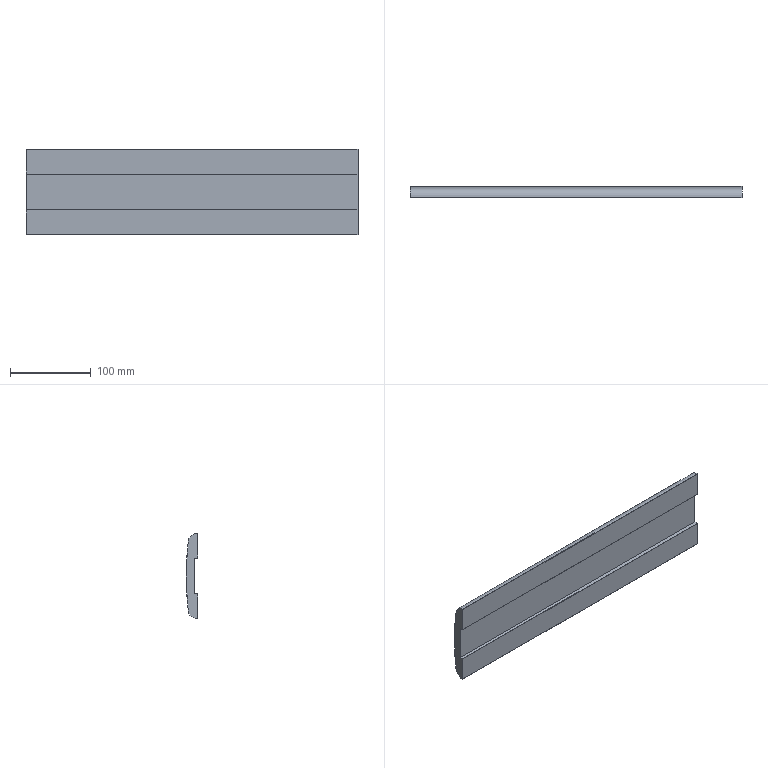Part | SolidWorks | features BaseBody 1 | 1 solid | 31 faces | box 411 x 14.5 x 106.047 mm | volume 473016 mm3 | cylinder 22 | plane 9 | commonest cylinder face diameters 0.2 x8 0.6 x6 22 x3 660 x3 0.4 x2
STEP:
#1=CARTESIAN_POINT('',(0.,60.288,-53.015));
#2=VERTEX_POINT('',#1);
#3=CARTESIAN_POINT('',(0.,60.72,-53.023));
#4=VERTEX_POINT('',#3);
#5=CARTESIAN_POINT('',(0.,60.72,-42.023));
#6=DIRECTION('',(1.,0.,0.));
#7=DIRECTION('',(0.,0.,-1.));
#8=AXIS2_PLACEMENT_3D('',#5,#6,#7);
#9=CIRCLE('',#8,11.);
#10=EDGE_CURVE('',#2,#4,#9,.T.);
#11=ORIENTED_EDGE('',*,*,#10,.T.);
#12=CARTESIAN_POINT('',(411.,60.72,-53.023));
#13=VERTEX_POINT('',#12);
#14=CARTESIAN_POINT('',(411.,60.72,-53.023));
#15=DIRECTION('',(1.,0.,0.));
#16=VECTOR('',#15,1000.);
#17=LINE('',#14,#16);
#18=EDGE_CURVE('',#4,#13,#17,.T.);
#19=ORIENTED_EDGE('',*,*,#18,.T.);
#20=CARTESIAN_POINT('',(411.,60.288,-53.015));
#21=VERTEX_POINT('',#20);
#22=CARTESIAN_POINT('',(411.,60.72,-42.023));
#23=DIRECTION('',(1.,0.,0.));
#24=DIRECTION('',(0.,0.,-1.));
#25=AXIS2_PLACEMENT_3D('',#22,#23,#24);
#26=CIRCLE('',#25,11.);
#27=EDGE_CURVE('',#21,#13,#26,.T.);
#28=ORIENTED_EDGE('',*,*,#27,.F.);
#29=CARTESIAN_POINT('',(411.,60.288,-53.015));
#30=DIRECTION('',(-1.,0.,0.));
#31=VECTOR('',#30,1000.);
#32=LINE('',#29,#31);
#33=EDGE_CURVE('',#21,#2,#32,.T.);
#34=ORIENTED_EDGE('',*,*,#33,.T.);
#35=EDGE_LOOP('',(#11,#19,#28,#34));
#36=FACE_OUTER_BOUND('',#35,.T.);
#37=CARTESIAN_POINT('',(411.,60.72,-42.023));
#38=DIRECTION('',(1.,0.,0.));
#39=DIRECTION('',(0.,0.,-1.));
#40=AXIS2_PLACEMENT_3D('',#37,#38,#39);
#41=CYLINDRICAL_SURFACE('',#40,11.);
#42=ADVANCED_FACE('',(#36),#41,.T.);
#43=CARTESIAN_POINT('',(411.,73.654,23.614));
#44=VERTEX_POINT('',#43);
#45=CARTESIAN_POINT('',(411.,73.654,-23.614));
#46=VERTEX_POINT('',#45);
#47=CARTESIAN_POINT('',(411.,-255.5,0.));
#48=DIRECTION('',(-1.,0.,0.));
#49=DIRECTION('',(0.,0.,-1.));
#50=AXIS2_PLACEMENT_3D('',#47,#48,#49);
#51=CIRCLE('',#50,330.);
#52=EDGE_CURVE('',#44,#46,#51,.T.);
#53=ORIENTED_EDGE('',*,*,#52,.T.);
#54=CARTESIAN_POINT('',(0.,73.654,-23.614));
#55=VERTEX_POINT('',#54);
#56=CARTESIAN_POINT('',(411.,73.654,-23.614));
#57=DIRECTION('',(-1.,0.,0.));
#58=VECTOR('',#57,1000.);
#59=LINE('',#56,#58);
#60=EDGE_CURVE('',#46,#55,#59,.T.);
#61=ORIENTED_EDGE('',*,*,#60,.T.);
#62=CARTESIAN_POINT('',(0.,73.654,23.614));
#63=VERTEX_POINT('',#62);
#64=CARTESIAN_POINT('',(0.,-255.5,0.));
#65=DIRECTION('',(1.,0.,0.));
#66=DIRECTION('',(0.,0.,-1.));
#67=AXIS2_PLACEMENT_3D('',#64,#65,#66);
#68=CIRCLE('',#67,330.);
#69=EDGE_CURVE('',#55,#63,#68,.T.);
#70=ORIENTED_EDGE('',*,*,#69,.T.);
#71=CARTESIAN_POINT('',(411.,73.654,23.614));
#72=DIRECTION('',(1.,0.,0.));
#73=VECTOR('',#72,1000.);
#74=LINE('',#71,#73);
#75=EDGE_CURVE('',#63,#44,#74,.T.);
#76=ORIENTED_EDGE('',*,*,#75,.T.);
#77=EDGE_LOOP('',(#53,#61,#70,#76));
#78=FACE_OUTER_BOUND('',#77,.T.);
#79=CARTESIAN_POINT('',(411.,-255.5,0.));
#80=DIRECTION('',(1.,0.,0.));
#81=DIRECTION('',(0.,0.,-1.));
#82=AXIS2_PLACEMENT_3D('',#79,#80,#81);
#83=CYLINDRICAL_SURFACE('',#82,330.);
#84=ADVANCED_FACE('',(#78),#83,.T.);
#85=CARTESIAN_POINT('',(411.,73.572,-23.705));
#86=VERTEX_POINT('',#85);
#87=CARTESIAN_POINT('',(411.,73.554,-23.607));
#88=DIRECTION('',(-1.,0.,0.));
#89=DIRECTION('',(0.,0.,-1.));
#90=AXIS2_PLACEMENT_3D('',#87,#88,#89);
#91=CIRCLE('',#90,0.1);
#92=EDGE_CURVE('',#46,#86,#91,.T.);
#93=ORIENTED_EDGE('',*,*,#92,.T.);
#94=CARTESIAN_POINT('',(0.,73.572,-23.705));
#95=VERTEX_POINT('',#94);
#96=CARTESIAN_POINT('',(411.,73.572,-23.705));
#97=DIRECTION('',(-1.,0.,0.));
#98=VECTOR('',#97,1000.);
#99=LINE('',#96,#98);
#100=EDGE_CURVE('',#86,#95,#99,.T.);
#101=ORIENTED_EDGE('',*,*,#100,.T.);
#102=CARTESIAN_POINT('',(0.,73.554,-23.607));
#103=DIRECTION('',(1.,0.,0.));
#104=DIRECTION('',(0.,0.,-1.));
#105=AXIS2_PLACEMENT_3D('',#102,#103,#104);
#106=CIRCLE('',#105,0.1);
#107=EDGE_CURVE('',#95,#55,#106,.T.);
#108=ORIENTED_EDGE('',*,*,#107,.T.);
#109=ORIENTED_EDGE('',*,*,#60,.F.);
#110=EDGE_LOOP('',(#93,#101,#108,#109));
#111=FACE_OUTER_BOUND('',#110,.T.);
#112=CARTESIAN_POINT('',(411.,73.554,-23.607));
#113=DIRECTION('',(1.,0.,0.));
#114=DIRECTION('',(0.,0.,-1.));
#115=AXIS2_PLACEMENT_3D('',#112,#113,#114);
#116=CYLINDRICAL_SURFACE('',#115,0.1);
#117=ADVANCED_FACE('',(#111),#116,.T.);
#118=CARTESIAN_POINT('',(411.,73.499,24.705));
#119=VERTEX_POINT('',#118);
#120=CARTESIAN_POINT('',(411.,73.455,25.284));
#121=VERTEX_POINT('',#120);
#122=CARTESIAN_POINT('',(411.,73.552,25.));
#123=DIRECTION('',(-1.,0.,0.));
#124=DIRECTION('',(0.,0.,-1.));
#125=AXIS2_PLACEMENT_3D('',#122,#123,#124);
#126=CIRCLE('',#125,0.3);
#127=EDGE_CURVE('',#119,#121,#126,.T.);
#128=ORIENTED_EDGE('',*,*,#127,.T.);
#129=CARTESIAN_POINT('',(411.,73.522,25.386));
#130=VERTEX_POINT('',#129);
#131=CARTESIAN_POINT('',(411.,73.422,25.378));
#132=DIRECTION('',(-1.,0.,0.));
#133=DIRECTION('',(0.,0.,-1.));
#134=AXIS2_PLACEMENT_3D('',#131,#132,#133);
#135=CIRCLE('',#134,0.1);
#136=EDGE_CURVE('',#130,#121,#135,.T.);
#137=ORIENTED_EDGE('',*,*,#136,.F.);
#138=CARTESIAN_POINT('',(411.,71.624,43.473));
#139=VERTEX_POINT('',#138);
#140=CARTESIAN_POINT('',(411.,-255.5,0.002391));
#141=DIRECTION('',(1.,0.,0.));
#142=DIRECTION('',(0.,0.,-1.));
#143=AXIS2_PLACEMENT_3D('',#140,#141,#142);
#144=CIRCLE('',#143,330.);
#145=EDGE_CURVE('',#130,#139,#144,.T.);
#146=ORIENTED_EDGE('',*,*,#145,.T.);
#147=CARTESIAN_POINT('',(411.,60.288,53.015));
#148=VERTEX_POINT('',#147);
#149=CARTESIAN_POINT('',(411.,60.72,42.023));
#150=DIRECTION('',(1.,0.,0.));
#151=DIRECTION('',(0.,0.,-1.));
#152=AXIS2_PLACEMENT_3D('',#149,#150,#151);
#153=CIRCLE('',#152,11.);
#154=EDGE_CURVE('',#139,#148,#153,.T.);
#155=ORIENTED_EDGE('',*,*,#154,.T.);
#156=CARTESIAN_POINT('',(411.,60.,52.715));
#157=VERTEX_POINT('',#156);
#158=CARTESIAN_POINT('',(411.,60.3,52.715));
#159=DIRECTION('',(-1.,0.,0.));
#160=DIRECTION('',(0.,0.,-1.));
#161=AXIS2_PLACEMENT_3D('',#158,#159,#160);
#162=CIRCLE('',#161,0.3);
#163=EDGE_CURVE('',#157,#148,#162,.T.);
#164=ORIENTED_EDGE('',*,*,#163,.F.);
#165=CARTESIAN_POINT('',(411.,60.,22.2));
#166=VERTEX_POINT('',#165);
#167=CARTESIAN_POINT('',(411.,60.,0.002391));
#168=DIRECTION('',(0.,0.,-1.));
#169=VECTOR('',#168,1000.);
#170=LINE('',#167,#169);
#171=EDGE_CURVE('',#157,#166,#170,.T.);
#172=ORIENTED_EDGE('',*,*,#171,.T.);
#173=CARTESIAN_POINT('',(411.,60.2,22.));
#174=VERTEX_POINT('',#173);
#175=CARTESIAN_POINT('',(411.,60.2,22.2));
#176=DIRECTION('',(-1.,0.,0.));
#177=DIRECTION('',(0.,0.,-1.));
#178=AXIS2_PLACEMENT_3D('',#175,#176,#177);
#179=CIRCLE('',#178,0.2);
#180=EDGE_CURVE('',#174,#166,#179,.T.);
#181=ORIENTED_EDGE('',*,*,#180,.F.);
#182=CARTESIAN_POINT('',(411.,64.5,22.));
#183=VERTEX_POINT('',#182);
#184=CARTESIAN_POINT('',(411.,-255.5,22.));
#185=DIRECTION('',(0.,1.,0.));
#186=VECTOR('',#185,1000.);
#187=LINE('',#184,#186);
#188=EDGE_CURVE('',#174,#183,#187,.T.);
#189=ORIENTED_EDGE('',*,*,#188,.T.);
#190=CARTESIAN_POINT('',(411.,64.5,-22.));
#191=VERTEX_POINT('',#190);
#192=CARTESIAN_POINT('',(411.,64.5,0.002391));
#193=DIRECTION('',(0.,0.,-1.));
#194=VECTOR('',#193,1000.);
#195=LINE('',#192,#194);
#196=EDGE_CURVE('',#183,#191,#195,.T.);
#197=ORIENTED_EDGE('',*,*,#196,.T.);
#198=CARTESIAN_POINT('',(411.,60.2,-22.));
#199=VERTEX_POINT('',#198);
#200=CARTESIAN_POINT('',(411.,-255.5,-22.));
#201=DIRECTION('',(0.,-1.,0.));
#202=VECTOR('',#201,1000.);
#203=LINE('',#200,#202);
#204=EDGE_CURVE('',#191,#199,#203,.T.);
#205=ORIENTED_EDGE('',*,*,#204,.T.);
#206=CARTESIAN_POINT('',(411.,60.,-22.2));
#207=VERTEX_POINT('',#206);
#208=CARTESIAN_POINT('',(411.,60.2,-22.2));
#209=DIRECTION('',(-1.,0.,0.));
#210=DIRECTION('',(0.,0.,-1.));
#211=AXIS2_PLACEMENT_3D('',#208,#209,#210);
#212=CIRCLE('',#211,0.2);
#213=EDGE_CURVE('',#207,#199,#212,.T.);
#214=ORIENTED_EDGE('',*,*,#213,.F.);
#215=CARTESIAN_POINT('',(411.,60.,-52.715));
#216=VERTEX_POINT('',#215);
#217=CARTESIAN_POINT('',(411.,60.,0.002391));
#218=DIRECTION('',(0.,0.,-1.));
#219=VECTOR('',#218,1000.);
#220=LINE('',#217,#219);
#221=EDGE_CURVE('',#207,#216,#220,.T.);
#222=ORIENTED_EDGE('',*,*,#221,.T.);
#223=CARTESIAN_POINT('',(411.,60.3,-52.715));
#224=DIRECTION('',(-1.,0.,0.));
#225=DIRECTION('',(0.,0.,-1.));
#226=AXIS2_PLACEMENT_3D('',#223,#224,#225);
#227=CIRCLE('',#226,0.3);
#228=EDGE_CURVE('',#21,#216,#227,.T.);
#229=ORIENTED_EDGE('',*,*,#228,.F.);
#230=ORIENTED_EDGE('',*,*,#27,.T.);
#231=CARTESIAN_POINT('',(411.,71.624,-43.473));
#232=VERTEX_POINT('',#231);
#233=CARTESIAN_POINT('',(411.,60.72,-42.023));
#234=DIRECTION('',(1.,0.,0.));
#235=DIRECTION('',(0.,0.,-1.));
#236=AXIS2_PLACEMENT_3D('',#233,#234,#235);
#237=CIRCLE('',#236,11.);
#238=EDGE_CURVE('',#13,#232,#237,.T.);
#239=ORIENTED_EDGE('',*,*,#238,.T.);
#240=CARTESIAN_POINT('',(411.,73.522,-25.386));
#241=VERTEX_POINT('',#240);
#242=CARTESIAN_POINT('',(411.,-255.5,-0.002391));
#243=DIRECTION('',(1.,0.,0.));
#244=DIRECTION('',(0.,0.,-1.));
#245=AXIS2_PLACEMENT_3D('',#242,#243,#244);
#246=CIRCLE('',#245,330.);
#247=EDGE_CURVE('',#232,#241,#246,.T.);
#248=ORIENTED_EDGE('',*,*,#247,.T.);
#249=CARTESIAN_POINT('',(411.,73.455,-25.284));
#250=VERTEX_POINT('',#249);
#251=CARTESIAN_POINT('',(411.,73.422,-25.378));
#252=DIRECTION('',(-1.,0.,0.));
#253=DIRECTION('',(0.,0.,-1.));
#254=AXIS2_PLACEMENT_3D('',#251,#252,#253);
#255=CIRCLE('',#254,0.1);
#256=EDGE_CURVE('',#250,#241,#255,.T.);
#257=ORIENTED_EDGE('',*,*,#256,.F.);
#258=CARTESIAN_POINT('',(411.,73.499,-24.705));
#259=VERTEX_POINT('',#258);
#260=CARTESIAN_POINT('',(411.,73.552,-25.));
#261=DIRECTION('',(-1.,0.,0.));
#262=DIRECTION('',(0.,0.,-1.));
#263=AXIS2_PLACEMENT_3D('',#260,#261,#262);
#264=CIRCLE('',#263,0.3);
#265=EDGE_CURVE('',#250,#259,#264,.T.);
#266=ORIENTED_EDGE('',*,*,#265,.T.);
#267=CARTESIAN_POINT('',(411.,73.581,-24.614));
#268=VERTEX_POINT('',#267);
#269=CARTESIAN_POINT('',(411.,73.481,-24.607));
#270=DIRECTION('',(-1.,0.,0.));
#271=DIRECTION('',(0.,0.,-1.));
#272=AXIS2_PLACEMENT_3D('',#269,#270,#271);
#273=CIRCLE('',#272,0.1);
#274=EDGE_CURVE('',#268,#259,#273,.T.);
#275=ORIENTED_EDGE('',*,*,#274,.F.);
#276=CARTESIAN_POINT('',(411.,73.598,-24.386));
#277=VERTEX_POINT('',#276);
#278=CARTESIAN_POINT('',(411.,73.581,-24.614));
#279=DIRECTION('',(0.,0.07436,0.9972));
#280=VECTOR('',#279,1000.);
#281=LINE('',#278,#280);
#282=EDGE_CURVE('',#268,#277,#281,.T.);
#283=ORIENTED_EDGE('',*,*,#282,.T.);
#284=CARTESIAN_POINT('',(411.,73.53,-24.284));
#285=VERTEX_POINT('',#284);
#286=CARTESIAN_POINT('',(411.,73.498,-24.379));
#287=DIRECTION('',(-1.,0.,0.));
#288=DIRECTION('',(0.,0.,-1.));
#289=AXIS2_PLACEMENT_3D('',#286,#287,#288);
#290=CIRCLE('',#289,0.1);
#291=EDGE_CURVE('',#285,#277,#290,.T.);
#292=ORIENTED_EDGE('',*,*,#291,.F.);
#293=CARTESIAN_POINT('',(411.,73.627,-24.));
#294=DIRECTION('',(-1.,0.,0.));
#295=DIRECTION('',(0.,0.,-1.));
#296=AXIS2_PLACEMENT_3D('',#293,#294,#295);
#297=CIRCLE('',#296,0.3);
#298=EDGE_CURVE('',#285,#86,#297,.T.);
#299=ORIENTED_EDGE('',*,*,#298,.T.);
#300=ORIENTED_EDGE('',*,*,#92,.F.);
#301=ORIENTED_EDGE('',*,*,#52,.F.);
#302=CARTESIAN_POINT('',(411.,73.572,23.705));
#303=VERTEX_POINT('',#302);
#304=CARTESIAN_POINT('',(411.,73.554,23.607));
#305=DIRECTION('',(1.,0.,0.));
#306=DIRECTION('',(0.,0.,-1.));
#307=AXIS2_PLACEMENT_3D('',#304,#305,#306);
#308=CIRCLE('',#307,0.1);
#309=EDGE_CURVE('',#44,#303,#308,.T.);
#310=ORIENTED_EDGE('',*,*,#309,.T.);
#311=CARTESIAN_POINT('',(411.,73.53,24.284));
#312=VERTEX_POINT('',#311);
#313=CARTESIAN_POINT('',(411.,73.627,24.));
#314=DIRECTION('',(-1.,0.,0.));
#315=DIRECTION('',(0.,0.,-1.));
#316=AXIS2_PLACEMENT_3D('',#313,#314,#315);
#317=CIRCLE('',#316,0.3);
#318=EDGE_CURVE('',#303,#312,#317,.T.);
#319=ORIENTED_EDGE('',*,*,#318,.T.);
#320=CARTESIAN_POINT('',(411.,73.598,24.386));
#321=VERTEX_POINT('',#320);
#322=CARTESIAN_POINT('',(411.,73.498,24.379));
#323=DIRECTION('',(-1.,0.,0.));
#324=DIRECTION('',(0.,0.,-1.));
#325=AXIS2_PLACEMENT_3D('',#322,#323,#324);
#326=CIRCLE('',#325,0.1);
#327=EDGE_CURVE('',#321,#312,#326,.T.);
#328=ORIENTED_EDGE('',*,*,#327,.F.);
#329=CARTESIAN_POINT('',(411.,73.581,24.614));
#330=VERTEX_POINT('',#329);
#331=CARTESIAN_POINT('',(411.,73.598,24.386));
#332=DIRECTION('',(0.,-0.07436,0.9972));
#333=VECTOR('',#332,1000.);
#334=LINE('',#331,#333);
#335=EDGE_CURVE('',#321,#330,#334,.T.);
#336=ORIENTED_EDGE('',*,*,#335,.T.);
#337=CARTESIAN_POINT('',(411.,73.481,24.607));
#338=DIRECTION('',(-1.,0.,0.));
#339=DIRECTION('',(0.,0.,-1.));
#340=AXIS2_PLACEMENT_3D('',#337,#338,#339);
#341=CIRCLE('',#340,0.1);
#342=EDGE_CURVE('',#119,#330,#341,.T.);
#343=ORIENTED_EDGE('',*,*,#342,.F.);
#344=EDGE_LOOP('',(#128,#137,#146,#155,#164,#172,#181,#189,#197,#205,#214,#222,#229,#230,#239,#248,#257,#266,#275,#283,#292,#299,#300,#301,#310,#319,#328,#336,#343));
#345=FACE_OUTER_BOUND('',#344,.T.);
#346=CARTESIAN_POINT('',(411.,-255.5,0.002391));
#347=DIRECTION('',(1.,0.,0.));
#348=DIRECTION('',(0.,0.,-1.));
#349=AXIS2_PLACEMENT_3D('',#346,#347,#348);
#350=PLANE('',#349);
#351=ADVANCED_FACE('',(#345),#350,.T.);
#352=ORIENTED_EDGE('',*,*,#309,.F.);
#353=ORIENTED_EDGE('',*,*,#75,.F.);
#354=CARTESIAN_POINT('',(0.,73.572,23.705));
#355=VERTEX_POINT('',#354);
#356=CARTESIAN_POINT('',(0.,73.554,23.607));
#357=DIRECTION('',(1.,0.,0.));
#358=DIRECTION('',(0.,0.,-1.));
#359=AXIS2_PLACEMENT_3D('',#356,#357,#358);
#360=CIRCLE('',#359,0.1);
#361=EDGE_CURVE('',#63,#355,#360,.T.);
#362=ORIENTED_EDGE('',*,*,#361,.T.);
#363=CARTESIAN_POINT('',(411.,73.572,23.705));
#364=DIRECTION('',(1.,0.,0.));
#365=VECTOR('',#364,1000.);
#366=LINE('',#363,#365);
#367=EDGE_CURVE('',#355,#303,#366,.T.);
#368=ORIENTED_EDGE('',*,*,#367,.T.);
#369=EDGE_LOOP('',(#352,#353,#362,#368));
#370=FACE_OUTER_BOUND('',#369,.T.);
#371=CARTESIAN_POINT('',(411.,73.554,23.607));
#372=DIRECTION('',(1.,0.,0.));
#373=DIRECTION('',(0.,0.,-1.));
#374=AXIS2_PLACEMENT_3D('',#371,#372,#373);
#375=CYLINDRICAL_SURFACE('',#374,0.1);
#376=ADVANCED_FACE('',(#370),#375,.T.);
#377=CARTESIAN_POINT('',(0.,73.455,25.284));
#378=VERTEX_POINT('',#377);
#379=CARTESIAN_POINT('',(0.,73.522,25.386));
#380=VERTEX_POINT('',#379);
#381=CARTESIAN_POINT('',(0.,73.422,25.378));
#382=DIRECTION('',(1.,0.,0.));
#383=DIRECTION('',(0.,0.,-1.));
#384=AXIS2_PLACEMENT_3D('',#381,#382,#383);
#385=CIRCLE('',#384,0.1);
#386=EDGE_CURVE('',#378,#380,#385,.T.);
#387=ORIENTED_EDGE('',*,*,#386,.F.);
#388=CARTESIAN_POINT('',(0.,73.499,24.705));
#389=VERTEX_POINT('',#388);
#390=CARTESIAN_POINT('',(0.,73.552,25.));
#391=DIRECTION('',(1.,0.,0.));
#392=DIRECTION('',(0.,0.,-1.));
#393=AXIS2_PLACEMENT_3D('',#390,#391,#392);
#394=CIRCLE('',#393,0.3);
#395=EDGE_CURVE('',#378,#389,#394,.T.);
#396=ORIENTED_EDGE('',*,*,#395,.T.);
#397=CARTESIAN_POINT('',(0.,73.581,24.614));
#398=VERTEX_POINT('',#397);
#399=CARTESIAN_POINT('',(0.,73.481,24.607));
#400=DIRECTION('',(1.,0.,0.));
#401=DIRECTION('',(0.,0.,-1.));
#402=AXIS2_PLACEMENT_3D('',#399,#400,#401);
#403=CIRCLE('',#402,0.1);
#404=EDGE_CURVE('',#398,#389,#403,.T.);
#405=ORIENTED_EDGE('',*,*,#404,.F.);
#406=CARTESIAN_POINT('',(0.,73.598,24.386));
#407=VERTEX_POINT('',#406);
#408=CARTESIAN_POINT('',(0.,73.598,24.386));
#409=DIRECTION('',(0.,0.07436,-0.9972));
#410=VECTOR('',#409,1000.);
#411=LINE('',#408,#410);
#412=EDGE_CURVE('',#398,#407,#411,.T.);
#413=ORIENTED_EDGE('',*,*,#412,.T.);
#414=CARTESIAN_POINT('',(0.,73.53,24.284));
#415=VERTEX_POINT('',#414);
#416=CARTESIAN_POINT('',(0.,73.498,24.379));
#417=DIRECTION('',(1.,0.,0.));
#418=DIRECTION('',(0.,0.,-1.));
#419=AXIS2_PLACEMENT_3D('',#416,#417,#418);
#420=CIRCLE('',#419,0.1);
#421=EDGE_CURVE('',#415,#407,#420,.T.);
#422=ORIENTED_EDGE('',*,*,#421,.F.);
#423=CARTESIAN_POINT('',(0.,73.627,24.));
#424=DIRECTION('',(-1.,0.,0.));
#425=DIRECTION('',(0.,0.,-1.));
#426=AXIS2_PLACEMENT_3D('',#423,#424,#425);
#427=CIRCLE('',#426,0.3);
#428=EDGE_CURVE('',#355,#415,#427,.T.);
#429=ORIENTED_EDGE('',*,*,#428,.F.);
#430=ORIENTED_EDGE('',*,*,#361,.F.);
#431=ORIENTED_EDGE('',*,*,#69,.F.);
#432=ORIENTED_EDGE('',*,*,#107,.F.);
#433=CARTESIAN_POINT('',(0.,73.53,-24.284));
#434=VERTEX_POINT('',#433);
#435=CARTESIAN_POINT('',(0.,73.627,-24.));
#436=DIRECTION('',(-1.,0.,0.));
#437=DIRECTION('',(0.,0.,-1.));
#438=AXIS2_PLACEMENT_3D('',#435,#436,#437);
#439=CIRCLE('',#438,0.3);
#440=EDGE_CURVE('',#434,#95,#439,.T.);
#441=ORIENTED_EDGE('',*,*,#440,.F.);
#442=CARTESIAN_POINT('',(0.,73.598,-24.386));
#443=VERTEX_POINT('',#442);
#444=CARTESIAN_POINT('',(0.,73.498,-24.379));
#445=DIRECTION('',(1.,0.,0.));
#446=DIRECTION('',(0.,0.,-1.));
#447=AXIS2_PLACEMENT_3D('',#444,#445,#446);
#448=CIRCLE('',#447,0.1);
#449=EDGE_CURVE('',#443,#434,#448,.T.);
#450=ORIENTED_EDGE('',*,*,#449,.F.);
#451=CARTESIAN_POINT('',(0.,73.581,-24.614));
#452=VERTEX_POINT('',#451);
#453=CARTESIAN_POINT('',(0.,73.581,-24.614));
#454=DIRECTION('',(0.,-0.07436,-0.9972));
#455=VECTOR('',#454,1000.);
#456=LINE('',#453,#455);
#457=EDGE_CURVE('',#443,#452,#456,.T.);
#458=ORIENTED_EDGE('',*,*,#457,.T.);
#459=CARTESIAN_POINT('',(0.,73.499,-24.705));
#460=VERTEX_POINT('',#459);
#461=CARTESIAN_POINT('',(0.,73.481,-24.607));
#462=DIRECTION('',(1.,0.,0.));
#463=DIRECTION('',(0.,0.,-1.));
#464=AXIS2_PLACEMENT_3D('',#461,#462,#463);
#465=CIRCLE('',#464,0.1);
#466=EDGE_CURVE('',#460,#452,#465,.T.);
#467=ORIENTED_EDGE('',*,*,#466,.F.);
#468=CARTESIAN_POINT('',(0.,73.455,-25.284));
#469=VERTEX_POINT('',#468);
#470=CARTESIAN_POINT('',(0.,73.552,-25.));
#471=DIRECTION('',(1.,0.,0.));
#472=DIRECTION('',(0.,0.,-1.));
#473=AXIS2_PLACEMENT_3D('',#470,#471,#472);
#474=CIRCLE('',#473,0.3);
#475=EDGE_CURVE('',#460,#469,#474,.T.);
#476=ORIENTED_EDGE('',*,*,#475,.T.);
#477=CARTESIAN_POINT('',(0.,73.522,-25.386));
#478=VERTEX_POINT('',#477);
#479=CARTESIAN_POINT('',(0.,73.422,-25.378));
#480=DIRECTION('',(1.,0.,0.));
#481=DIRECTION('',(0.,0.,-1.));
#482=AXIS2_PLACEMENT_3D('',#479,#480,#481);
#483=CIRCLE('',#482,0.1);
#484=EDGE_CURVE('',#478,#469,#483,.T.);
#485=ORIENTED_EDGE('',*,*,#484,.F.);
#486=CARTESIAN_POINT('',(0.,71.624,-43.473));
#487=VERTEX_POINT('',#486);
#488=CARTESIAN_POINT('',(0.,-255.5,-0.002391));
#489=DIRECTION('',(1.,0.,0.));
#490=DIRECTION('',(0.,0.,-1.));
#491=AXIS2_PLACEMENT_3D('',#488,#489,#490);
#492=CIRCLE('',#491,330.);
#493=EDGE_CURVE('',#487,#478,#492,.T.);
#494=ORIENTED_EDGE('',*,*,#493,.F.);
#495=CARTESIAN_POINT('',(0.,60.72,-42.023));
#496=DIRECTION('',(1.,0.,0.));
#497=DIRECTION('',(0.,0.,-1.));
#498=AXIS2_PLACEMENT_3D('',#495,#496,#497);
#499=CIRCLE('',#498,11.);
#500=EDGE_CURVE('',#4,#487,#499,.T.);
#501=ORIENTED_EDGE('',*,*,#500,.F.);
#502=ORIENTED_EDGE('',*,*,#10,.F.);
#503=CARTESIAN_POINT('',(0.,60.,-52.715));
#504=VERTEX_POINT('',#503);
#505=CARTESIAN_POINT('',(0.,60.3,-52.715));
#506=DIRECTION('',(1.,0.,0.));
#507=DIRECTION('',(0.,0.,-1.));
#508=AXIS2_PLACEMENT_3D('',#505,#506,#507);
#509=CIRCLE('',#508,0.3);
#510=EDGE_CURVE('',#504,#2,#509,.T.);
#511=ORIENTED_EDGE('',*,*,#510,.F.);
#512=CARTESIAN_POINT('',(0.,60.,-22.2));
#513=VERTEX_POINT('',#512);
#514=CARTESIAN_POINT('',(0.,60.,0.002391));
#515=DIRECTION('',(0.,0.,-1.));
#516=VECTOR('',#515,1000.);
#517=LINE('',#514,#516);
#518=EDGE_CURVE('',#513,#504,#517,.T.);
#519=ORIENTED_EDGE('',*,*,#518,.F.);
#520=CARTESIAN_POINT('',(0.,60.2,-22.));
#521=VERTEX_POINT('',#520);
#522=CARTESIAN_POINT('',(0.,60.2,-22.2));
#523=DIRECTION('',(1.,0.,0.));
#524=DIRECTION('',(0.,0.,-1.));
#525=AXIS2_PLACEMENT_3D('',#522,#523,#524);
#526=CIRCLE('',#525,0.2);
#527=EDGE_CURVE('',#521,#513,#526,.T.);
#528=ORIENTED_EDGE('',*,*,#527,.F.);
#529=CARTESIAN_POINT('',(0.,64.5,-22.));
#530=VERTEX_POINT('',#529);
#531=CARTESIAN_POINT('',(0.,-255.5,-22.));
#532=DIRECTION('',(0.,-1.,0.));
#533=VECTOR('',#532,1000.);
#534=LINE('',#531,#533);
#535=EDGE_CURVE('',#530,#521,#534,.T.);
#536=ORIENTED_EDGE('',*,*,#535,.F.);
#537=CARTESIAN_POINT('',(0.,64.5,22.));
#538=VERTEX_POINT('',#537);
#539=CARTESIAN_POINT('',(0.,64.5,0.002391));
#540=DIRECTION('',(0.,0.,-1.));
#541=VECTOR('',#540,1000.);
#542=LINE('',#539,#541);
#543=EDGE_CURVE('',#538,#530,#542,.T.);
#544=ORIENTED_EDGE('',*,*,#543,.F.);
#545=CARTESIAN_POINT('',(0.,60.2,22.));
#546=VERTEX_POINT('',#545);
#547=CARTESIAN_POINT('',(0.,-255.5,22.));
#548=DIRECTION('',(0.,1.,0.));
#549=VECTOR('',#548,1000.);
#550=LINE('',#547,#549);
#551=EDGE_CURVE('',#546,#538,#550,.T.);
#552=ORIENTED_EDGE('',*,*,#551,.F.);
#553=CARTESIAN_POINT('',(0.,60.,22.2));
#554=VERTEX_POINT('',#553);
#555=CARTESIAN_POINT('',(0.,60.2,22.2));
#556=DIRECTION('',(1.,0.,0.));
#557=DIRECTION('',(0.,0.,-1.));
#558=AXIS2_PLACEMENT_3D('',#555,#556,#557);
#559=CIRCLE('',#558,0.2);
#560=EDGE_CURVE('',#554,#546,#559,.T.);
#561=ORIENTED_EDGE('',*,*,#560,.F.);
#562=CARTESIAN_POINT('',(0.,60.,52.715));
#563=VERTEX_POINT('',#562);
#564=CARTESIAN_POINT('',(0.,60.,0.002391));
#565=DIRECTION('',(0.,0.,-1.));
#566=VECTOR('',#565,1000.);
#567=LINE('',#564,#566);
#568=EDGE_CURVE('',#563,#554,#567,.T.);
#569=ORIENTED_EDGE('',*,*,#568,.F.);
#570=CARTESIAN_POINT('',(0.,60.288,53.015));
#571=VERTEX_POINT('',#570);
#572=CARTESIAN_POINT('',(0.,60.3,52.715));
#573=DIRECTION('',(1.,0.,0.));
#574=DIRECTION('',(0.,0.,-1.));
#575=AXIS2_PLACEMENT_3D('',#572,#573,#574);
#576=CIRCLE('',#575,0.3);
#577=EDGE_CURVE('',#571,#563,#576,.T.);
#578=ORIENTED_EDGE('',*,*,#577,.F.);
#579=CARTESIAN_POINT('',(0.,71.624,43.473));
#580=VERTEX_POINT('',#579);
#581=CARTESIAN_POINT('',(0.,60.72,42.023));
#582=DIRECTION('',(1.,0.,0.));
#583=DIRECTION('',(0.,0.,-1.));
#584=AXIS2_PLACEMENT_3D('',#581,#582,#583);
#585=CIRCLE('',#584,11.);
#586=EDGE_CURVE('',#580,#571,#585,.T.);
#587=ORIENTED_EDGE('',*,*,#586,.F.);
#588=CARTESIAN_POINT('',(0.,-255.5,0.002391));
#589=DIRECTION('',(1.,0.,0.));
#590=DIRECTION('',(0.,0.,-1.));
#591=AXIS2_PLACEMENT_3D('',#588,#589,#590);
#592=CIRCLE('',#591,330.);
#593=EDGE_CURVE('',#380,#580,#592,.T.);
#594=ORIENTED_EDGE('',*,*,#593,.F.);
#595=EDGE_LOOP('',(#387,#396,#405,#413,#422,#429,#430,#431,#432,#441,#450,#458,#467,#476,#485,#494,#501,#502,#511,#519,#528,#536,#544,#552,#561,#569,#578,#587,#594));
#596=FACE_OUTER_BOUND('',#595,.T.);
#597=CARTESIAN_POINT('',(0.,-255.5,0.002391));
#598=DIRECTION('',(1.,0.,0.));
#599=DIRECTION('',(0.,0.,-1.));
#600=AXIS2_PLACEMENT_3D('',#597,#598,#599);
#601=PLANE('',#600);
#602=ADVANCED_FACE('',(#596),#601,.F.);
#603=ORIENTED_EDGE('',*,*,#100,.F.);
#604=ORIENTED_EDGE('',*,*,#298,.F.);
#605=CARTESIAN_POINT('',(411.,73.53,-24.284));
#606=DIRECTION('',(1.,0.,0.));
#607=VECTOR('',#606,1000.);
#608=LINE('',#605,#607);
#609=EDGE_CURVE('',#434,#285,#608,.T.);
#610=ORIENTED_EDGE('',*,*,#609,.F.);
#611=ORIENTED_EDGE('',*,*,#440,.T.);
#612=EDGE_LOOP('',(#603,#604,#610,#611));
#613=FACE_OUTER_BOUND('',#612,.T.);
#614=CARTESIAN_POINT('',(411.,73.627,-24.));
#615=DIRECTION('',(1.,0.,0.));
#616=DIRECTION('',(0.,0.,-1.));
#617=AXIS2_PLACEMENT_3D('',#614,#615,#616);
#618=CYLINDRICAL_SURFACE('',#617,0.3);
#619=ADVANCED_FACE('',(#613),#618,.F.);
#620=ORIENTED_EDGE('',*,*,#247,.F.);
#621=CARTESIAN_POINT('',(411.,71.624,-43.473));
#622=DIRECTION('',(-1.,0.,0.));
#623=VECTOR('',#622,1000.);
#624=LINE('',#621,#623);
#625=EDGE_CURVE('',#232,#487,#624,.T.);
#626=ORIENTED_EDGE('',*,*,#625,.T.);
#627=ORIENTED_EDGE('',*,*,#493,.T.);
#628=CARTESIAN_POINT('',(411.,73.522,-25.386));
#629=DIRECTION('',(1.,0.,0.));
#630=VECTOR('',#629,1000.);
#631=LINE('',#628,#630);
#632=EDGE_CURVE('',#478,#241,#631,.T.);
#633=ORIENTED_EDGE('',*,*,#632,.T.);
#634=EDGE_LOOP('',(#620,#626,#627,#633));
#635=FACE_OUTER_BOUND('',#634,.T.);
#636=CARTESIAN_POINT('',(411.,-255.5,-0.002391));
#637=DIRECTION('',(1.,0.,0.));
#638=DIRECTION('',(0.,0.,-1.));
#639=AXIS2_PLACEMENT_3D('',#636,#637,#638);
#640=CYLINDRICAL_SURFACE('',#639,330.);
#641=ADVANCED_FACE('',(#635),#640,.T.);
#642=ORIENTED_EDGE('',*,*,#18,.F.);
#643=ORIENTED_EDGE('',*,*,#500,.T.);
#644=ORIENTED_EDGE('',*,*,#625,.F.);
#645=ORIENTED_EDGE('',*,*,#238,.F.);
#646=EDGE_LOOP('',(#642,#643,#644,#645));
#647=FACE_OUTER_BOUND('',#646,.T.);
#648=CARTESIAN_POINT('',(411.,60.72,-42.023));
#649=DIRECTION('',(1.,0.,0.));
#650=DIRECTION('',(0.,0.,-1.));
#651=AXIS2_PLACEMENT_3D('',#648,#649,#650);
#652=CYLINDRICAL_SURFACE('',#651,11.);
#653=ADVANCED_FACE('',(#647),#652,.T.);
#654=CARTESIAN_POINT('',(411.,60.,-52.715));
#655=DIRECTION('',(-1.,0.,0.));
#656=VECTOR('',#655,1000.);
#657=LINE('',#654,#656);
#658=EDGE_CURVE('',#216,#504,#657,.T.);
#659=ORIENTED_EDGE('',*,*,#658,.F.);
#660=ORIENTED_EDGE('',*,*,#221,.F.);
#661=CARTESIAN_POINT('',(411.,60.,-22.2));
#662=DIRECTION('',(1.,0.,0.));
#663=VECTOR('',#662,1000.);
#664=LINE('',#661,#663);
#665=EDGE_CURVE('',#513,#207,#664,.T.);
#666=ORIENTED_EDGE('',*,*,#665,.F.);
#667=ORIENTED_EDGE('',*,*,#518,.T.);
#668=EDGE_LOOP('',(#659,#660,#666,#667));
#669=FACE_OUTER_BOUND('',#668,.T.);
#670=CARTESIAN_POINT('',(411.,60.,-22.2));
#671=DIRECTION('',(0.,1.,0.));
#672=DIRECTION('',(0.,0.,1.));
#673=AXIS2_PLACEMENT_3D('',#670,#671,#672);
#674=PLANE('',#673);
#675=ADVANCED_FACE('',(#669),#674,.F.);
#676=CARTESIAN_POINT('',(411.,60.2,-22.));
#677=DIRECTION('',(-1.,0.,0.));
#678=VECTOR('',#677,1000.);
#679=LINE('',#676,#678);
#680=EDGE_CURVE('',#199,#521,#679,.T.);
#681=ORIENTED_EDGE('',*,*,#680,.F.);
#682=ORIENTED_EDGE('',*,*,#204,.F.);
#683=CARTESIAN_POINT('',(411.,64.5,-22.));
#684=DIRECTION('',(1.,0.,0.));
#685=VECTOR('',#684,1000.);
#686=LINE('',#683,#685);
#687=EDGE_CURVE('',#530,#191,#686,.T.);
#688=ORIENTED_EDGE('',*,*,#687,.F.);
#689=ORIENTED_EDGE('',*,*,#535,.T.);
#690=EDGE_LOOP('',(#681,#682,#688,#689));
#691=FACE_OUTER_BOUND('',#690,.T.);
#692=CARTESIAN_POINT('',(411.,64.5,-22.));
#693=DIRECTION('',(0.,0.,-1.));
#694=DIRECTION('',(-1.,0.,0.));
#695=AXIS2_PLACEMENT_3D('',#692,#693,#694);
#696=PLANE('',#695);
#697=ADVANCED_FACE('',(#691),#696,.F.);
#698=ORIENTED_EDGE('',*,*,#687,.T.);
#699=ORIENTED_EDGE('',*,*,#196,.F.);
#700=CARTESIAN_POINT('',(411.,64.5,22.));
#701=DIRECTION('',(1.,0.,0.));
#702=VECTOR('',#701,1000.);
#703=LINE('',#700,#702);
#704=EDGE_CURVE('',#538,#183,#703,.T.);
#705=ORIENTED_EDGE('',*,*,#704,.F.);
#706=ORIENTED_EDGE('',*,*,#543,.T.);
#707=EDGE_LOOP('',(#698,#699,#705,#706));
#708=FACE_OUTER_BOUND('',#707,.T.);
#709=CARTESIAN_POINT('',(411.,64.5,22.));
#710=DIRECTION('',(0.,1.,0.));
#711=DIRECTION('',(0.,0.,1.));
#712=AXIS2_PLACEMENT_3D('',#709,#710,#711);
#713=PLANE('',#712);
#714=ADVANCED_FACE('',(#708),#713,.F.);
#715=ORIENTED_EDGE('',*,*,#704,.T.);
#716=ORIENTED_EDGE('',*,*,#188,.F.);
#717=CARTESIAN_POINT('',(411.,60.2,22.));
#718=DIRECTION('',(1.,0.,0.));
#719=VECTOR('',#718,1000.);
#720=LINE('',#717,#719);
#721=EDGE_CURVE('',#546,#174,#720,.T.);
#722=ORIENTED_EDGE('',*,*,#721,.F.);
#723=ORIENTED_EDGE('',*,*,#551,.T.);
#724=EDGE_LOOP('',(#715,#716,#722,#723));
#725=FACE_OUTER_BOUND('',#724,.T.);
#726=CARTESIAN_POINT('',(411.,60.2,22.));
#727=DIRECTION('',(0.,0.,1.));
#728=DIRECTION('',(1.,0.,0.));
#729=AXIS2_PLACEMENT_3D('',#726,#727,#728);
#730=PLANE('',#729);
#731=ADVANCED_FACE('',(#725),#730,.F.);
#732=CARTESIAN_POINT('',(411.,60.,22.2));
#733=DIRECTION('',(-1.,0.,0.));
#734=VECTOR('',#733,1000.);
#735=LINE('',#732,#734);
#736=EDGE_CURVE('',#166,#554,#735,.T.);
#737=ORIENTED_EDGE('',*,*,#736,.F.);
#738=ORIENTED_EDGE('',*,*,#171,.F.);
#739=CARTESIAN_POINT('',(411.,60.,52.715));
#740=DIRECTION('',(1.,0.,0.));
#741=VECTOR('',#740,1000.);
#742=LINE('',#739,#741);
#743=EDGE_CURVE('',#563,#157,#742,.T.);
#744=ORIENTED_EDGE('',*,*,#743,.F.);
#745=ORIENTED_EDGE('',*,*,#568,.T.);
#746=EDGE_LOOP('',(#737,#738,#744,#745));
#747=FACE_OUTER_BOUND('',#746,.T.);
#748=CARTESIAN_POINT('',(411.,60.,52.715));
#749=DIRECTION('',(0.,1.,0.));
#750=DIRECTION('',(0.,0.,1.));
#751=AXIS2_PLACEMENT_3D('',#748,#749,#750);
#752=PLANE('',#751);
#753=ADVANCED_FACE('',(#747),#752,.F.);
#754=ORIENTED_EDGE('',*,*,#154,.F.);
#755=CARTESIAN_POINT('',(411.,71.624,43.473));
#756=DIRECTION('',(-1.,0.,0.));
#757=VECTOR('',#756,1000.);
#758=LINE('',#755,#757);
#759=EDGE_CURVE('',#139,#580,#758,.T.);
#760=ORIENTED_EDGE('',*,*,#759,.T.);
#761=ORIENTED_EDGE('',*,*,#586,.T.);
#762=CARTESIAN_POINT('',(411.,60.288,53.015));
#763=DIRECTION('',(1.,0.,0.));
#764=VECTOR('',#763,1000.);
#765=LINE('',#762,#764);
#766=EDGE_CURVE('',#571,#148,#765,.T.);
#767=ORIENTED_EDGE('',*,*,#766,.T.);
#768=EDGE_LOOP('',(#754,#760,#761,#767));
#769=FACE_OUTER_BOUND('',#768,.T.);
#770=CARTESIAN_POINT('',(411.,60.72,42.023));
#771=DIRECTION('',(1.,0.,0.));
#772=DIRECTION('',(0.,0.,-1.));
#773=AXIS2_PLACEMENT_3D('',#770,#771,#772);
#774=CYLINDRICAL_SURFACE('',#773,11.);
#775=ADVANCED_FACE('',(#769),#774,.T.);
#776=ORIENTED_EDGE('',*,*,#145,.F.);
#777=CARTESIAN_POINT('',(411.,73.522,25.386));
#778=DIRECTION('',(-1.,0.,0.));
#779=VECTOR('',#778,1000.);
#780=LINE('',#777,#779);
#781=EDGE_CURVE('',#130,#380,#780,.T.);
#782=ORIENTED_EDGE('',*,*,#781,.T.);
#783=ORIENTED_EDGE('',*,*,#593,.T.);
#784=ORIENTED_EDGE('',*,*,#759,.F.);
#785=EDGE_LOOP('',(#776,#782,#783,#784));
#786=FACE_OUTER_BOUND('',#785,.T.);
#787=CARTESIAN_POINT('',(411.,-255.5,0.002391));
#788=DIRECTION('',(1.,0.,0.));
#789=DIRECTION('',(0.,0.,-1.));
#790=AXIS2_PLACEMENT_3D('',#787,#788,#789);
#791=CYLINDRICAL_SURFACE('',#790,330.);
#792=ADVANCED_FACE('',(#786),#791,.T.);
#793=CARTESIAN_POINT('',(411.,73.53,24.284));
#794=DIRECTION('',(-1.,0.,0.));
#795=VECTOR('',#794,1000.);
#796=LINE('',#793,#795);
#797=EDGE_CURVE('',#312,#415,#796,.T.);
#798=ORIENTED_EDGE('',*,*,#797,.F.);
#799=ORIENTED_EDGE('',*,*,#318,.F.);
#800=ORIENTED_EDGE('',*,*,#367,.F.);
#801=ORIENTED_EDGE('',*,*,#428,.T.);
#802=EDGE_LOOP('',(#798,#799,#800,#801));
#803=FACE_OUTER_BOUND('',#802,.T.);
#804=CARTESIAN_POINT('',(411.,73.627,24.));
#805=DIRECTION('',(1.,0.,0.));
#806=DIRECTION('',(0.,0.,-1.));
#807=AXIS2_PLACEMENT_3D('',#804,#805,#806);
#808=CYLINDRICAL_SURFACE('',#807,0.3);
#809=ADVANCED_FACE('',(#803),#808,.F.);
#810=ORIENTED_EDGE('',*,*,#291,.T.);
#811=CARTESIAN_POINT('',(411.,73.598,-24.386));
#812=DIRECTION('',(-1.,0.,0.));
#813=VECTOR('',#812,1000.);
#814=LINE('',#811,#813);
#815=EDGE_CURVE('',#277,#443,#814,.T.);
#816=ORIENTED_EDGE('',*,*,#815,.T.);
#817=ORIENTED_EDGE('',*,*,#449,.T.);
#818=ORIENTED_EDGE('',*,*,#609,.T.);
#819=EDGE_LOOP('',(#810,#816,#817,#818));
#820=FACE_OUTER_BOUND('',#819,.T.);
#821=CARTESIAN_POINT('',(411.,73.498,-24.379));
#822=DIRECTION('',(1.,0.,0.));
#823=DIRECTION('',(0.,0.,-1.));
#824=AXIS2_PLACEMENT_3D('',#821,#822,#823);
#825=CYLINDRICAL_SURFACE('',#824,0.1);
#826=ADVANCED_FACE('',(#820),#825,.T.);
#827=ORIENTED_EDGE('',*,*,#256,.T.);
#828=ORIENTED_EDGE('',*,*,#632,.F.);
#829=ORIENTED_EDGE('',*,*,#484,.T.);
#830=CARTESIAN_POINT('',(411.,73.455,-25.284));
#831=DIRECTION('',(1.,0.,0.));
#832=VECTOR('',#831,1000.);
#833=LINE('',#830,#832);
#834=EDGE_CURVE('',#469,#250,#833,.T.);
#835=ORIENTED_EDGE('',*,*,#834,.T.);
#836=EDGE_LOOP('',(#827,#828,#829,#835));
#837=FACE_OUTER_BOUND('',#836,.T.);
#838=CARTESIAN_POINT('',(411.,73.422,-25.378));
#839=DIRECTION('',(1.,0.,0.));
#840=DIRECTION('',(0.,0.,-1.));
#841=AXIS2_PLACEMENT_3D('',#838,#839,#840);
#842=CYLINDRICAL_SURFACE('',#841,0.1);
#843=ADVANCED_FACE('',(#837),#842,.T.);
#844=ORIENTED_EDGE('',*,*,#228,.T.);
#845=ORIENTED_EDGE('',*,*,#658,.T.);
#846=ORIENTED_EDGE('',*,*,#510,.T.);
#847=ORIENTED_EDGE('',*,*,#33,.F.);
#848=EDGE_LOOP('',(#844,#845,#846,#847));
#849=FACE_OUTER_BOUND('',#848,.T.);
#850=CARTESIAN_POINT('',(411.,60.3,-52.715));
#851=DIRECTION('',(1.,0.,0.));
#852=DIRECTION('',(0.,0.,-1.));
#853=AXIS2_PLACEMENT_3D('',#850,#851,#852);
#854=CYLINDRICAL_SURFACE('',#853,0.3);
#855=ADVANCED_FACE('',(#849),#854,.T.);
#856=ORIENTED_EDGE('',*,*,#213,.T.);
#857=ORIENTED_EDGE('',*,*,#680,.T.);
#858=ORIENTED_EDGE('',*,*,#527,.T.);
#859=ORIENTED_EDGE('',*,*,#665,.T.);
#860=EDGE_LOOP('',(#856,#857,#858,#859));
#861=FACE_OUTER_BOUND('',#860,.T.);
#862=CARTESIAN_POINT('',(411.,60.2,-22.2));
#863=DIRECTION('',(1.,0.,0.));
#864=DIRECTION('',(0.,0.,-1.));
#865=AXIS2_PLACEMENT_3D('',#862,#863,#864);
#866=CYLINDRICAL_SURFACE('',#865,0.2);
#867=ADVANCED_FACE('',(#861),#866,.T.);
#868=ORIENTED_EDGE('',*,*,#180,.T.);
#869=ORIENTED_EDGE('',*,*,#736,.T.);
#870=ORIENTED_EDGE('',*,*,#560,.T.);
#871=ORIENTED_EDGE('',*,*,#721,.T.);
#872=EDGE_LOOP('',(#868,#869,#870,#871));
#873=FACE_OUTER_BOUND('',#872,.T.);
#874=CARTESIAN_POINT('',(411.,60.2,22.2));
#875=DIRECTION('',(1.,0.,0.));
#876=DIRECTION('',(0.,0.,-1.));
#877=AXIS2_PLACEMENT_3D('',#874,#875,#876);
#878=CYLINDRICAL_SURFACE('',#877,0.2);
#879=ADVANCED_FACE('',(#873),#878,.T.);
#880=ORIENTED_EDGE('',*,*,#163,.T.);
#881=ORIENTED_EDGE('',*,*,#766,.F.);
#882=ORIENTED_EDGE('',*,*,#577,.T.);
#883=ORIENTED_EDGE('',*,*,#743,.T.);
#884=EDGE_LOOP('',(#880,#881,#882,#883));
#885=FACE_OUTER_BOUND('',#884,.T.);
#886=CARTESIAN_POINT('',(411.,60.3,52.715));
#887=DIRECTION('',(1.,0.,0.));
#888=DIRECTION('',(0.,0.,-1.));
#889=AXIS2_PLACEMENT_3D('',#886,#887,#888);
#890=CYLINDRICAL_SURFACE('',#889,0.3);
#891=ADVANCED_FACE('',(#885),#890,.T.);
#892=ORIENTED_EDGE('',*,*,#136,.T.);
#893=CARTESIAN_POINT('',(411.,73.455,25.284));
#894=DIRECTION('',(-1.,0.,0.));
#895=VECTOR('',#894,1000.);
#896=LINE('',#893,#895);
#897=EDGE_CURVE('',#121,#378,#896,.T.);
#898=ORIENTED_EDGE('',*,*,#897,.T.);
#899=ORIENTED_EDGE('',*,*,#386,.T.);
#900=ORIENTED_EDGE('',*,*,#781,.F.);
#901=EDGE_LOOP('',(#892,#898,#899,#900));
#902=FACE_OUTER_BOUND('',#901,.T.);
#903=CARTESIAN_POINT('',(411.,73.422,25.378));
#904=DIRECTION('',(1.,0.,0.));
#905=DIRECTION('',(0.,0.,-1.));
#906=AXIS2_PLACEMENT_3D('',#903,#904,#905);
#907=CYLINDRICAL_SURFACE('',#906,0.1);
#908=ADVANCED_FACE('',(#902),#907,.T.);
#909=ORIENTED_EDGE('',*,*,#327,.T.);
#910=ORIENTED_EDGE('',*,*,#797,.T.);
#911=ORIENTED_EDGE('',*,*,#421,.T.);
#912=CARTESIAN_POINT('',(411.,73.598,24.386));
#913=DIRECTION('',(1.,0.,0.));
#914=VECTOR('',#913,1000.);
#915=LINE('',#912,#914);
#916=EDGE_CURVE('',#407,#321,#915,.T.);
#917=ORIENTED_EDGE('',*,*,#916,.T.);
#918=EDGE_LOOP('',(#909,#910,#911,#917));
#919=FACE_OUTER_BOUND('',#918,.T.);
#920=CARTESIAN_POINT('',(411.,73.498,24.379));
#921=DIRECTION('',(1.,0.,0.));
#922=DIRECTION('',(0.,0.,-1.));
#923=AXIS2_PLACEMENT_3D('',#920,#921,#922);
#924=CYLINDRICAL_SURFACE('',#923,0.1);
#925=ADVANCED_FACE('',(#919),#924,.T.);
#926=ORIENTED_EDGE('',*,*,#815,.F.);
#927=ORIENTED_EDGE('',*,*,#282,.F.);
#928=CARTESIAN_POINT('',(411.,73.581,-24.614));
#929=DIRECTION('',(1.,0.,0.));
#930=VECTOR('',#929,1000.);
#931=LINE('',#928,#930);
#932=EDGE_CURVE('',#452,#268,#931,.T.);
#933=ORIENTED_EDGE('',*,*,#932,.F.);
#934=ORIENTED_EDGE('',*,*,#457,.F.);
#935=EDGE_LOOP('',(#926,#927,#933,#934));
#936=FACE_OUTER_BOUND('',#935,.T.);
#937=CARTESIAN_POINT('',(411.,73.581,-24.614));
#938=DIRECTION('',(0.,-0.9972,0.07436));
#939=DIRECTION('',(0.,-0.07436,-0.9972));
#940=AXIS2_PLACEMENT_3D('',#937,#938,#939);
#941=PLANE('',#940);
#942=ADVANCED_FACE('',(#936),#941,.F.);
#943=CARTESIAN_POINT('',(411.,73.499,-24.705));
#944=DIRECTION('',(-1.,0.,0.));
#945=VECTOR('',#944,1000.);
#946=LINE('',#943,#945);
#947=EDGE_CURVE('',#259,#460,#946,.T.);
#948=ORIENTED_EDGE('',*,*,#947,.F.);
#949=ORIENTED_EDGE('',*,*,#265,.F.);
#950=ORIENTED_EDGE('',*,*,#834,.F.);
#951=ORIENTED_EDGE('',*,*,#475,.F.);
#952=EDGE_LOOP('',(#948,#949,#950,#951));
#953=FACE_OUTER_BOUND('',#952,.T.);
#954=CARTESIAN_POINT('',(411.,73.552,-25.));
#955=DIRECTION('',(1.,0.,0.));
#956=DIRECTION('',(0.,0.,-1.));
#957=AXIS2_PLACEMENT_3D('',#954,#955,#956);
#958=CYLINDRICAL_SURFACE('',#957,0.3);
#959=ADVANCED_FACE('',(#953),#958,.F.);
#960=ORIENTED_EDGE('',*,*,#897,.F.);
#961=ORIENTED_EDGE('',*,*,#127,.F.);
#962=CARTESIAN_POINT('',(411.,73.499,24.705));
#963=DIRECTION('',(1.,0.,0.));
#964=VECTOR('',#963,1000.);
#965=LINE('',#962,#964);
#966=EDGE_CURVE('',#389,#119,#965,.T.);
#967=ORIENTED_EDGE('',*,*,#966,.F.);
#968=ORIENTED_EDGE('',*,*,#395,.F.);
#969=EDGE_LOOP('',(#960,#961,#967,#968));
#970=FACE_OUTER_BOUND('',#969,.T.);
#971=CARTESIAN_POINT('',(411.,73.552,25.));
#972=DIRECTION('',(1.,0.,0.));
#973=DIRECTION('',(0.,0.,-1.));
#974=AXIS2_PLACEMENT_3D('',#971,#972,#973);
#975=CYLINDRICAL_SURFACE('',#974,0.3);
#976=ADVANCED_FACE('',(#970),#975,.F.);
#977=CARTESIAN_POINT('',(411.,73.581,24.614));
#978=DIRECTION('',(-1.,0.,0.));
#979=VECTOR('',#978,1000.);
#980=LINE('',#977,#979);
#981=EDGE_CURVE('',#330,#398,#980,.T.);
#982=ORIENTED_EDGE('',*,*,#981,.F.);
#983=ORIENTED_EDGE('',*,*,#335,.F.);
#984=ORIENTED_EDGE('',*,*,#916,.F.);
#985=ORIENTED_EDGE('',*,*,#412,.F.);
#986=EDGE_LOOP('',(#982,#983,#984,#985));
#987=FACE_OUTER_BOUND('',#986,.T.);
#988=CARTESIAN_POINT('',(411.,73.598,24.386));
#989=DIRECTION('',(0.,-0.9972,-0.07436));
#990=DIRECTION('',(0.,0.07436,-0.9972));
#991=AXIS2_PLACEMENT_3D('',#988,#989,#990);
#992=PLANE('',#991);
#993=ADVANCED_FACE('',(#987),#992,.F.);
#994=ORIENTED_EDGE('',*,*,#274,.T.);
#995=ORIENTED_EDGE('',*,*,#947,.T.);
#996=ORIENTED_EDGE('',*,*,#466,.T.);
#997=ORIENTED_EDGE('',*,*,#932,.T.);
#998=EDGE_LOOP('',(#994,#995,#996,#997));
#999=FACE_OUTER_BOUND('',#998,.T.);
#1000=CARTESIAN_POINT('',(411.,73.481,-24.607));
#1001=DIRECTION('',(1.,0.,0.));
#1002=DIRECTION('',(0.,0.,-1.));
#1003=AXIS2_PLACEMENT_3D('',#1000,#1001,#1002);
#1004=CYLINDRICAL_SURFACE('',#1003,0.1);
#1005=ADVANCED_FACE('',(#999),#1004,.T.);
#1006=ORIENTED_EDGE('',*,*,#342,.T.);
#1007=ORIENTED_EDGE('',*,*,#981,.T.);
#1008=ORIENTED_EDGE('',*,*,#404,.T.);
#1009=ORIENTED_EDGE('',*,*,#966,.T.);
#1010=EDGE_LOOP('',(#1006,#1007,#1008,#1009));
#1011=FACE_OUTER_BOUND('',#1010,.T.);
#1012=CARTESIAN_POINT('',(411.,73.481,24.607));
#1013=DIRECTION('',(1.,0.,0.));
#1014=DIRECTION('',(0.,0.,-1.));
#1015=AXIS2_PLACEMENT_3D('',#1012,#1013,#1014);
#1016=CYLINDRICAL_SURFACE('',#1015,0.1);
#1017=ADVANCED_FACE('',(#1011),#1016,.T.);
#1018=CLOSED_SHELL('',(#42,#84,#117,#351,#376,#602,#619,#641,#653,#675,#697,#714,#731,#753,#775,#792,#809,#826,#843,#855,#867,#879,#891,#908,#925,#942,#959,#976,#993,#1005,#1017));
#1019=MANIFOLD_SOLID_BREP('',#1018);
#1020=CARTESIAN_POINT('',(0.,0.,0.));
#1021=DIRECTION('',(0.,0.,1.));
#1022=DIRECTION('',(1.,0.,0.));
#1023=AXIS2_PLACEMENT_3D('',#1020,#1021,#1022);
#1024=(LENGTH_UNIT()NAMED_UNIT(*)SI_UNIT(.MILLI.,.METRE.));
#1025=UNCERTAINTY_MEASURE_WITH_UNIT(LENGTH_MEASURE(0.00001),#1024,'','');
#1026=(NAMED_UNIT(*)PLANE_ANGLE_UNIT()SI_UNIT($,.RADIAN.));
#1027=(NAMED_UNIT(*)SI_UNIT($,.STERADIAN.)SOLID_ANGLE_UNIT());
#1028=(GEOMETRIC_REPRESENTATION_CONTEXT(3)GLOBAL_UNCERTAINTY_ASSIGNED_CONTEXT((#1025))GLOBAL_UNIT_ASSIGNED_CONTEXT((#1024,#1026,#1027))REPRESENTATION_CONTEXT('',''));
#1029=ADVANCED_BREP_SHAPE_REPRESENTATION('',(#1019,#1023),#1028);